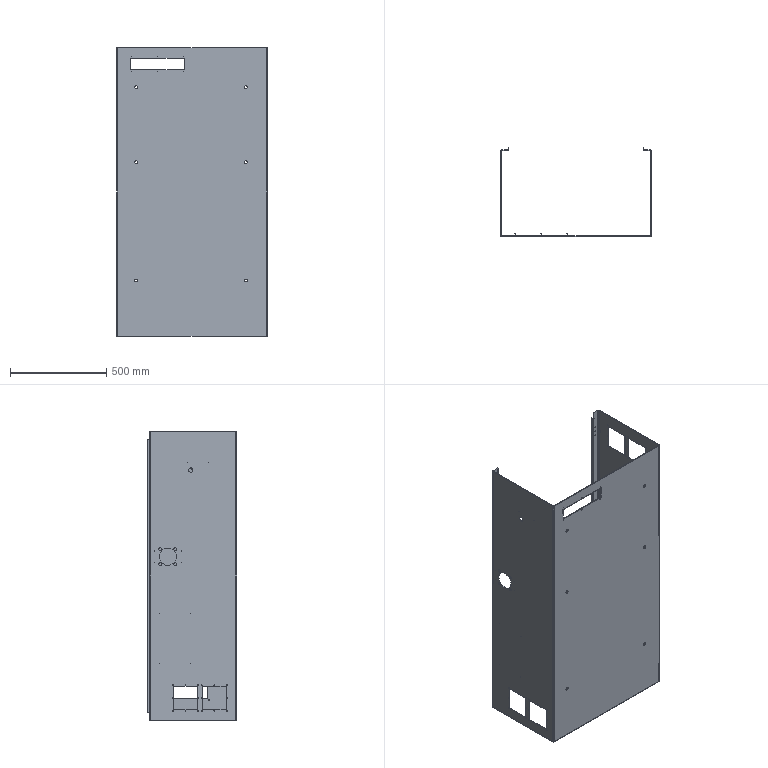Part | NX | features solid 2 | 1 solid | 261 faces | box 780 x 463.5 x 1500 mm | volume 5071499 mm3 | cylinder 200 | plane 61 | commonest cylinder face diameters 5 x82 1 x62 15 x20 6.2 x8 4 x6 6 x6